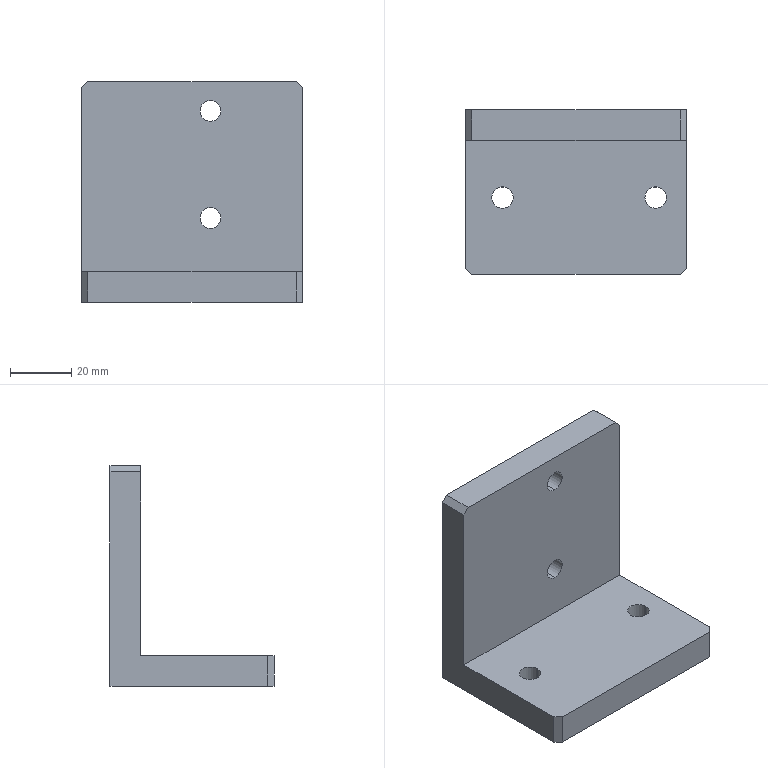Part | STEP file | Cable Carrier Bracket 3 | 1 solid | 20 faces | box 72 x 53.558 x 72 mm | volume 81626 mm3 | plane 12 | cylinder 8 | commonest cylinder face diameters 6.8 x4 7 x4